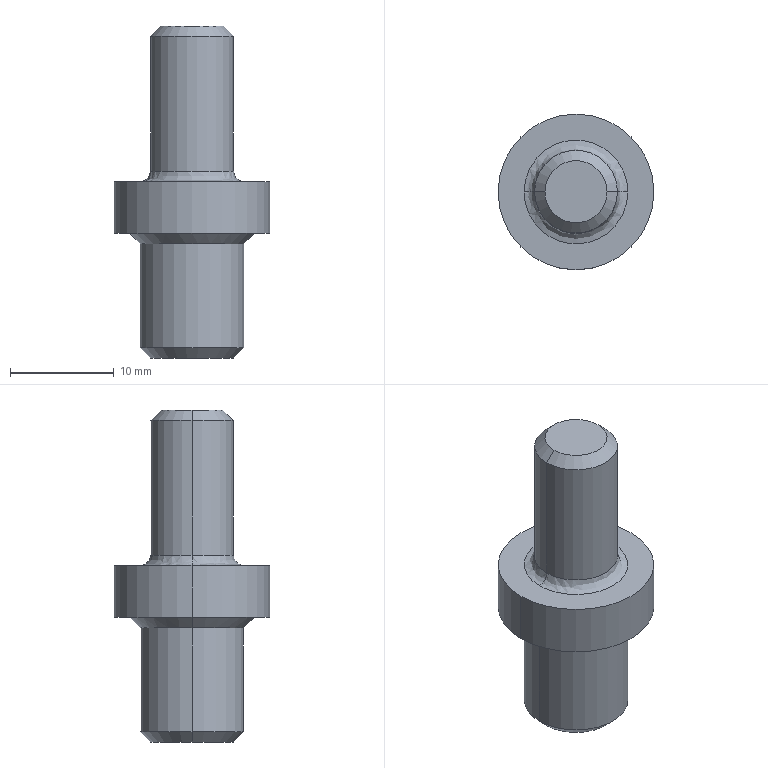Part | SolidWorks | features BaseBody 1 | 1 solid | 18 faces | box 15 x 15 x 32 mm | volume 2576 mm3 | cylinder 6 | cone 6 | plane 4 | spline 2 | commonest cylinder face diameters 8 x2 10 x2 15 x2
STEP:
#1=CARTESIAN_POINT('',(-5.,0.,5.));
#2=VERTEX_POINT('',#1);
#3=CARTESIAN_POINT('',(5.,0.,5.));
#4=VERTEX_POINT('',#3);
#5=CARTESIAN_POINT('',(-5.,0.,5.));
#6=CARTESIAN_POINT('',(-5.,0.3177,5.));
#7=CARTESIAN_POINT('',(-4.956,0.7861,5.));
#8=CARTESIAN_POINT('',(-4.828,1.318,5.));
#9=CARTESIAN_POINT('',(-4.745,1.58,5.));
#10=CARTESIAN_POINT('',(-4.699,1.711,5.));
#11=CARTESIAN_POINT('',(-4.678,1.766,5.));
#12=CARTESIAN_POINT('',(-4.663,1.803,5.));
#13=CARTESIAN_POINT('',(-4.657,1.821,5.));
#14=CARTESIAN_POINT('',(-4.587,1.997,5.));
#15=CARTESIAN_POINT('',(-4.482,2.227,5.));
#16=CARTESIAN_POINT('',(-4.361,2.448,5.));
#17=CARTESIAN_POINT('',(-4.276,2.594,5.));
#18=CARTESIAN_POINT('',(-4.232,2.664,5.));
#19=CARTESIAN_POINT('',(-3.996,3.025,5.));
#20=CARTESIAN_POINT('',(-3.779,3.292,5.));
#21=CARTESIAN_POINT('',(-3.414,3.657,5.));
#22=CARTESIAN_POINT('',(-3.222,3.83,5.));
#23=CARTESIAN_POINT('',(-3.018,3.987,5.));
#24=CARTESIAN_POINT('',(-2.879,4.089,5.));
#25=CARTESIAN_POINT('',(-2.807,4.139,5.));
#26=CARTESIAN_POINT('',(-2.595,4.277,5.));
#27=CARTESIAN_POINT('',(-2.377,4.405,5.));
#28=CARTESIAN_POINT('',(-2.112,4.533,5.));
#29=CARTESIAN_POINT('',(-1.977,4.593,5.));
#30=CARTESIAN_POINT('',(-1.919,4.617,5.));
#31=CARTESIAN_POINT('',(-1.88,4.633,5.));
#32=CARTESIAN_POINT('',(-1.859,4.642,5.));
#33=CARTESIAN_POINT('',(-1.25,4.883,5.));
#34=CARTESIAN_POINT('',(-0.6355,5.,5.));
#35=CARTESIAN_POINT('',(0.3177,5.,5.));
#36=CARTESIAN_POINT('',(0.7861,4.956,5.));
#37=CARTESIAN_POINT('',(1.318,4.828,5.));
#38=CARTESIAN_POINT('',(1.58,4.745,5.));
#39=CARTESIAN_POINT('',(1.711,4.699,5.));
#40=CARTESIAN_POINT('',(1.766,4.678,5.));
#41=CARTESIAN_POINT('',(1.803,4.663,5.));
#42=CARTESIAN_POINT('',(1.821,4.657,5.));
#43=CARTESIAN_POINT('',(1.997,4.587,5.));
#44=CARTESIAN_POINT('',(2.227,4.482,5.));
#45=CARTESIAN_POINT('',(2.448,4.361,5.));
#46=CARTESIAN_POINT('',(2.594,4.276,5.));
#47=CARTESIAN_POINT('',(2.664,4.232,5.));
#48=CARTESIAN_POINT('',(3.025,3.996,5.));
#49=CARTESIAN_POINT('',(3.292,3.779,5.));
#50=CARTESIAN_POINT('',(3.657,3.414,5.));
#51=CARTESIAN_POINT('',(3.83,3.222,5.));
#52=CARTESIAN_POINT('',(3.987,3.018,5.));
#53=CARTESIAN_POINT('',(4.089,2.879,5.));
#54=CARTESIAN_POINT('',(4.139,2.807,5.));
#55=CARTESIAN_POINT('',(4.277,2.595,5.));
#56=CARTESIAN_POINT('',(4.405,2.377,5.));
#57=CARTESIAN_POINT('',(4.533,2.112,5.));
#58=CARTESIAN_POINT('',(4.584,1.996,5.));
#59=CARTESIAN_POINT('',(4.617,1.919,5.));
#60=CARTESIAN_POINT('',(4.634,1.878,5.));
#61=CARTESIAN_POINT('',(4.709,1.69,5.));
#62=CARTESIAN_POINT('',(4.787,1.461,5.));
#63=CARTESIAN_POINT('',(4.858,1.187,5.));
#64=CARTESIAN_POINT('',(4.889,1.049,5.));
#65=CARTESIAN_POINT('',(4.901,0.9894,5.));
#66=CARTESIAN_POINT('',(4.909,0.9497,5.));
#67=CARTESIAN_POINT('',(4.913,0.9286,5.));
#68=CARTESIAN_POINT('',(4.972,0.6093,5.));
#69=CARTESIAN_POINT('',(5.,0.306,5.));
#70=CARTESIAN_POINT('',(5.,0.,5.));
#71=B_SPLINE_CURVE_WITH_KNOTS('',3,(#5,#6,#7,#8,#9,#10,#11,#12,#13,#14,#15,#16,#17,#18,#19,#20,#21,#22,#23,#24,#25,#26,#27,#28,#29,#30,#31,#32,#33,#34,#35,#36,#37,#38,#39,#40,#41,#42,#43,#44,#45,#46,#47,#48,#49,#50,#51,#52,#53,#54,#55,#56,#57,#58,#59,#60,#61,#62,#63,#64,#65,#66,#67,#68,#69,#70),.UNSPECIFIED.,.F.,.F.,(4,1,1,1,1,2,2,1,2,2,2,1,2,2,1,1,1,2,2,2,1,1,1,1,2,2,1,2,2,2,1,2,2,1,1,2,2,1,1,1,2,2,4),(0.5,0.5313,0.5469,0.5547,0.5586,0.5605,0.5625,0.5781,0.5859,0.5938,0.625,0.6406,0.6484,0.6562,0.6719,0.6797,0.6836,0.6855,0.6875,0.75,0.7812,0.7969,0.8047,0.8086,0.8105,0.8125,0.8281,0.8359,0.8437,0.875,0.8906,0.8984,0.9062,0.9219,0.9297,0.9336,0.9375,0.9531,0.9609,0.9648,0.9668,0.9687,1.),.UNSPECIFIED.);
#72=EDGE_CURVE('',#2,#4,#71,.T.);
#73=ORIENTED_EDGE('',*,*,#72,.F.);
#74=CARTESIAN_POINT('',(-4.,0.,6.));
#75=VERTEX_POINT('',#74);
#76=CARTESIAN_POINT('',(-5.,0.,6.));
#77=DIRECTION('',(0.,-1.,0.));
#78=DIRECTION('',(-1.,0.,0.));
#79=AXIS2_PLACEMENT_3D('',#76,#77,#78);
#80=CIRCLE('',#79,1.);
#81=EDGE_CURVE('',#2,#75,#80,.T.);
#82=ORIENTED_EDGE('',*,*,#81,.T.);
#83=CARTESIAN_POINT('',(4.,0.,6.));
#84=VERTEX_POINT('',#83);
#85=CARTESIAN_POINT('',(0.,0.,6.));
#86=DIRECTION('',(0.,0.,1.));
#87=DIRECTION('',(-1.,0.,0.));
#88=AXIS2_PLACEMENT_3D('',#85,#86,#87);
#89=CIRCLE('',#88,4.);
#90=EDGE_CURVE('',#84,#75,#89,.T.);
#91=ORIENTED_EDGE('',*,*,#90,.F.);
#92=CARTESIAN_POINT('',(5.,0.,6.));
#93=DIRECTION('',(0.,1.,0.));
#94=DIRECTION('',(1.,0.,0.));
#95=AXIS2_PLACEMENT_3D('',#92,#93,#94);
#96=CIRCLE('',#95,1.);
#97=EDGE_CURVE('',#4,#84,#96,.T.);
#98=ORIENTED_EDGE('',*,*,#97,.F.);
#99=EDGE_LOOP('',(#73,#82,#91,#98));
#100=FACE_OUTER_BOUND('',#99,.T.);
#101=CARTESIAN_POINT('',(5.,0.,5.));
#102=CARTESIAN_POINT('',(5.,10.,5.));
#103=CARTESIAN_POINT('',(-5.,10.,5.));
#104=CARTESIAN_POINT('',(-5.,0.,5.));
#105=CARTESIAN_POINT('',(4.414,0.,5.));
#106=CARTESIAN_POINT('',(4.414,8.828,5.));
#107=CARTESIAN_POINT('',(-4.414,8.828,5.));
#108=CARTESIAN_POINT('',(-4.414,0.,5.));
#109=CARTESIAN_POINT('',(4.,0.,5.414));
#110=CARTESIAN_POINT('',(4.,8.,5.414));
#111=CARTESIAN_POINT('',(-4.,8.,5.414));
#112=CARTESIAN_POINT('',(-4.,0.,5.414));
#113=CARTESIAN_POINT('',(4.,0.,6.));
#114=CARTESIAN_POINT('',(4.,8.,6.));
#115=CARTESIAN_POINT('',(-4.,8.,6.));
#116=CARTESIAN_POINT('',(-4.,0.,6.));
#117=(BOUNDED_SURFACE()B_SPLINE_SURFACE(3,3,((#101,#102,#103,#104),(#105,#106,#107,#108),(#109,#110,#111,#112),(#113,#114,#115,#116)),.UNSPECIFIED.,.F.,.F.,.F.)B_SPLINE_SURFACE_WITH_KNOTS((4,4),(4,4),(0.,1.),(0.,1.),.UNSPECIFIED.)GEOMETRIC_REPRESENTATION_ITEM()RATIONAL_B_SPLINE_SURFACE(((1.,0.3333,0.3333,1.),(0.8047,0.2682,0.2682,0.8047),(0.8047,0.2682,0.2682,0.8047),(1.,0.3333,0.3333,1.)))REPRESENTATION_ITEM('')SURFACE());
#118=ADVANCED_FACE('',(#100),#117,.F.);
#119=CARTESIAN_POINT('',(-4.,0.,19.));
#120=VERTEX_POINT('',#119);
#121=CARTESIAN_POINT('',(4.,0.,19.));
#122=VERTEX_POINT('',#121);
#123=CARTESIAN_POINT('',(0.,0.,19.));
#124=DIRECTION('',(0.,0.,-1.));
#125=DIRECTION('',(-1.,0.,0.));
#126=AXIS2_PLACEMENT_3D('',#123,#124,#125);
#127=CIRCLE('',#126,4.);
#128=EDGE_CURVE('',#120,#122,#127,.T.);
#129=ORIENTED_EDGE('',*,*,#128,.T.);
#130=CARTESIAN_POINT('',(4.,0.,20.));
#131=DIRECTION('',(0.,0.,-1.));
#132=VECTOR('',#131,1000.);
#133=LINE('',#130,#132);
#134=EDGE_CURVE('',#122,#84,#133,.T.);
#135=ORIENTED_EDGE('',*,*,#134,.T.);
#136=ORIENTED_EDGE('',*,*,#90,.T.);
#137=CARTESIAN_POINT('',(-4.,0.,20.));
#138=DIRECTION('',(0.,0.,-1.));
#139=VECTOR('',#138,1000.);
#140=LINE('',#137,#139);
#141=EDGE_CURVE('',#120,#75,#140,.T.);
#142=ORIENTED_EDGE('',*,*,#141,.F.);
#143=EDGE_LOOP('',(#129,#135,#136,#142));
#144=FACE_OUTER_BOUND('',#143,.T.);
#145=CARTESIAN_POINT('',(0.,0.,20.));
#146=DIRECTION('',(0.,0.,-1.));
#147=DIRECTION('',(-1.,0.,0.));
#148=AXIS2_PLACEMENT_3D('',#145,#146,#147);
#149=CYLINDRICAL_SURFACE('',#148,4.);
#150=ADVANCED_FACE('',(#144),#149,.T.);
#151=CARTESIAN_POINT('',(-3.,0.,20.));
#152=VERTEX_POINT('',#151);
#153=CARTESIAN_POINT('',(3.,0.,20.));
#154=VERTEX_POINT('',#153);
#155=CARTESIAN_POINT('',(0.,0.,20.));
#156=DIRECTION('',(0.,0.,-1.));
#157=DIRECTION('',(-1.,0.,0.));
#158=AXIS2_PLACEMENT_3D('',#155,#156,#157);
#159=CIRCLE('',#158,3.);
#160=EDGE_CURVE('',#152,#154,#159,.T.);
#161=ORIENTED_EDGE('',*,*,#160,.T.);
#162=CARTESIAN_POINT('',(4.,0.,19.));
#163=DIRECTION('',(0.7071,0.,-0.7071));
#164=VECTOR('',#163,1000.);
#165=LINE('',#162,#164);
#166=EDGE_CURVE('',#154,#122,#165,.T.);
#167=ORIENTED_EDGE('',*,*,#166,.T.);
#168=ORIENTED_EDGE('',*,*,#128,.F.);
#169=CARTESIAN_POINT('',(-4.,0.,19.));
#170=DIRECTION('',(-0.7071,0.,-0.7071));
#171=VECTOR('',#170,1000.);
#172=LINE('',#169,#171);
#173=EDGE_CURVE('',#152,#120,#172,.T.);
#174=ORIENTED_EDGE('',*,*,#173,.F.);
#175=EDGE_LOOP('',(#161,#167,#168,#174));
#176=FACE_OUTER_BOUND('',#175,.T.);
#177=CARTESIAN_POINT('',(0.,0.,19.));
#178=DIRECTION('',(0.,0.,-1.));
#179=DIRECTION('',(-1.,0.,0.));
#180=AXIS2_PLACEMENT_3D('',#177,#178,#179);
#181=CONICAL_SURFACE('',#180,4.,0.7854);
#182=ADVANCED_FACE('',(#176),#181,.T.);
#183=CARTESIAN_POINT('',(7.5,0.,5.));
#184=VERTEX_POINT('',#183);
#185=CARTESIAN_POINT('',(-7.5,0.,5.));
#186=VERTEX_POINT('',#185);
#187=CARTESIAN_POINT('',(0.,0.,5.));
#188=DIRECTION('',(0.,0.,1.));
#189=DIRECTION('',(-1.,0.,0.));
#190=AXIS2_PLACEMENT_3D('',#187,#188,#189);
#191=CIRCLE('',#190,7.5);
#192=EDGE_CURVE('',#184,#186,#191,.T.);
#193=ORIENTED_EDGE('',*,*,#192,.F.);
#194=CARTESIAN_POINT('',(7.5,0.,0.));
#195=VERTEX_POINT('',#194);
#196=CARTESIAN_POINT('',(7.5,0.,5.));
#197=DIRECTION('',(0.,0.,-1.));
#198=VECTOR('',#197,1000.);
#199=LINE('',#196,#198);
#200=EDGE_CURVE('',#184,#195,#199,.T.);
#201=ORIENTED_EDGE('',*,*,#200,.T.);
#202=CARTESIAN_POINT('',(-7.5,0.,0.));
#203=VERTEX_POINT('',#202);
#204=CARTESIAN_POINT('',(0.,0.,0.));
#205=DIRECTION('',(0.,0.,1.));
#206=DIRECTION('',(-1.,0.,0.));
#207=AXIS2_PLACEMENT_3D('',#204,#205,#206);
#208=CIRCLE('',#207,7.5);
#209=EDGE_CURVE('',#195,#203,#208,.T.);
#210=ORIENTED_EDGE('',*,*,#209,.T.);
#211=CARTESIAN_POINT('',(-7.5,0.,5.));
#212=DIRECTION('',(0.,0.,-1.));
#213=VECTOR('',#212,1000.);
#214=LINE('',#211,#213);
#215=EDGE_CURVE('',#186,#203,#214,.T.);
#216=ORIENTED_EDGE('',*,*,#215,.F.);
#217=EDGE_LOOP('',(#193,#201,#210,#216));
#218=FACE_OUTER_BOUND('',#217,.T.);
#219=CARTESIAN_POINT('',(0.,0.,5.));
#220=DIRECTION('',(0.,0.,-1.));
#221=DIRECTION('',(-1.,0.,0.));
#222=AXIS2_PLACEMENT_3D('',#219,#220,#221);
#223=CYLINDRICAL_SURFACE('',#222,7.5);
#224=ADVANCED_FACE('',(#218),#223,.T.);
#225=CARTESIAN_POINT('',(5.,0.,-1.));
#226=VERTEX_POINT('',#225);
#227=CARTESIAN_POINT('',(-5.,0.,-1.));
#228=VERTEX_POINT('',#227);
#229=CARTESIAN_POINT('',(0.,0.,-1.));
#230=DIRECTION('',(0.,0.,1.));
#231=DIRECTION('',(1.,0.,0.));
#232=AXIS2_PLACEMENT_3D('',#229,#230,#231);
#233=CIRCLE('',#232,5.);
#234=EDGE_CURVE('',#226,#228,#233,.T.);
#235=ORIENTED_EDGE('',*,*,#234,.T.);
#236=CARTESIAN_POINT('',(-6.,0.,0.));
#237=VERTEX_POINT('',#236);
#238=CARTESIAN_POINT('',(-6.,0.,0.));
#239=DIRECTION('',(-0.7071,0.,0.7071));
#240=VECTOR('',#239,1000.);
#241=LINE('',#238,#240);
#242=EDGE_CURVE('',#228,#237,#241,.T.);
#243=ORIENTED_EDGE('',*,*,#242,.T.);
#244=CARTESIAN_POINT('',(6.,0.,0.));
#245=VERTEX_POINT('',#244);
#246=CARTESIAN_POINT('',(0.,0.,0.));
#247=DIRECTION('',(0.,0.,-1.));
#248=DIRECTION('',(1.,0.,0.));
#249=AXIS2_PLACEMENT_3D('',#246,#247,#248);
#250=CIRCLE('',#249,6.);
#251=EDGE_CURVE('',#237,#245,#250,.T.);
#252=ORIENTED_EDGE('',*,*,#251,.T.);
#253=CARTESIAN_POINT('',(6.,0.,0.));
#254=DIRECTION('',(0.7071,0.,0.7071));
#255=VECTOR('',#254,1000.);
#256=LINE('',#253,#255);
#257=EDGE_CURVE('',#226,#245,#256,.T.);
#258=ORIENTED_EDGE('',*,*,#257,.F.);
#259=EDGE_LOOP('',(#235,#243,#252,#258));
#260=FACE_OUTER_BOUND('',#259,.T.);
#261=CARTESIAN_POINT('',(0.,0.,0.));
#262=DIRECTION('',(0.,0.,1.));
#263=DIRECTION('',(1.,0.,0.));
#264=AXIS2_PLACEMENT_3D('',#261,#262,#263);
#265=CONICAL_SURFACE('',#264,6.,0.7854);
#266=ADVANCED_FACE('',(#260),#265,.T.);
#267=CARTESIAN_POINT('',(5.,0.,-11.));
#268=VERTEX_POINT('',#267);
#269=CARTESIAN_POINT('',(-5.,0.,-11.));
#270=VERTEX_POINT('',#269);
#271=CARTESIAN_POINT('',(0.,0.,-11.));
#272=DIRECTION('',(0.,0.,1.));
#273=DIRECTION('',(1.,0.,0.));
#274=AXIS2_PLACEMENT_3D('',#271,#272,#273);
#275=CIRCLE('',#274,5.);
#276=EDGE_CURVE('',#268,#270,#275,.T.);
#277=ORIENTED_EDGE('',*,*,#276,.T.);
#278=CARTESIAN_POINT('',(-5.,0.,-12.));
#279=DIRECTION('',(0.,0.,1.));
#280=VECTOR('',#279,1000.);
#281=LINE('',#278,#280);
#282=EDGE_CURVE('',#270,#228,#281,.T.);
#283=ORIENTED_EDGE('',*,*,#282,.T.);
#284=ORIENTED_EDGE('',*,*,#234,.F.);
#285=CARTESIAN_POINT('',(5.,0.,-12.));
#286=DIRECTION('',(0.,0.,1.));
#287=VECTOR('',#286,1000.);
#288=LINE('',#285,#287);
#289=EDGE_CURVE('',#268,#226,#288,.T.);
#290=ORIENTED_EDGE('',*,*,#289,.F.);
#291=EDGE_LOOP('',(#277,#283,#284,#290));
#292=FACE_OUTER_BOUND('',#291,.T.);
#293=CARTESIAN_POINT('',(0.,0.,-12.));
#294=DIRECTION('',(0.,0.,1.));
#295=DIRECTION('',(1.,0.,0.));
#296=AXIS2_PLACEMENT_3D('',#293,#294,#295);
#297=CYLINDRICAL_SURFACE('',#296,5.);
#298=ADVANCED_FACE('',(#292),#297,.T.);
#299=CARTESIAN_POINT('',(4.,0.,-12.));
#300=VERTEX_POINT('',#299);
#301=CARTESIAN_POINT('',(-4.,0.,-12.));
#302=VERTEX_POINT('',#301);
#303=CARTESIAN_POINT('',(0.,0.,-12.));
#304=DIRECTION('',(0.,0.,1.));
#305=DIRECTION('',(1.,0.,0.));
#306=AXIS2_PLACEMENT_3D('',#303,#304,#305);
#307=CIRCLE('',#306,4.);
#308=EDGE_CURVE('',#300,#302,#307,.T.);
#309=ORIENTED_EDGE('',*,*,#308,.T.);
#310=CARTESIAN_POINT('',(-5.,0.,-11.));
#311=DIRECTION('',(-0.7071,0.,0.7071));
#312=VECTOR('',#311,1000.);
#313=LINE('',#310,#312);
#314=EDGE_CURVE('',#302,#270,#313,.T.);
#315=ORIENTED_EDGE('',*,*,#314,.T.);
#316=ORIENTED_EDGE('',*,*,#276,.F.);
#317=CARTESIAN_POINT('',(5.,0.,-11.));
#318=DIRECTION('',(0.7071,0.,0.7071));
#319=VECTOR('',#318,1000.);
#320=LINE('',#317,#319);
#321=EDGE_CURVE('',#300,#268,#320,.T.);
#322=ORIENTED_EDGE('',*,*,#321,.F.);
#323=EDGE_LOOP('',(#309,#315,#316,#322));
#324=FACE_OUTER_BOUND('',#323,.T.);
#325=CARTESIAN_POINT('',(0.,0.,-11.));
#326=DIRECTION('',(0.,0.,1.));
#327=DIRECTION('',(1.,0.,0.));
#328=AXIS2_PLACEMENT_3D('',#325,#326,#327);
#329=CONICAL_SURFACE('',#328,5.,0.7854);
#330=ADVANCED_FACE('',(#324),#329,.T.);
#331=ORIENTED_EDGE('',*,*,#134,.F.);
#332=CARTESIAN_POINT('',(0.,0.,19.));
#333=DIRECTION('',(0.,0.,-1.));
#334=DIRECTION('',(-1.,0.,0.));
#335=AXIS2_PLACEMENT_3D('',#332,#333,#334);
#336=CIRCLE('',#335,4.);
#337=EDGE_CURVE('',#122,#120,#336,.T.);
#338=ORIENTED_EDGE('',*,*,#337,.T.);
#339=ORIENTED_EDGE('',*,*,#141,.T.);
#340=CARTESIAN_POINT('',(0.,0.,6.));
#341=DIRECTION('',(0.,0.,1.));
#342=DIRECTION('',(-1.,0.,0.));
#343=AXIS2_PLACEMENT_3D('',#340,#341,#342);
#344=CIRCLE('',#343,4.);
#345=EDGE_CURVE('',#75,#84,#344,.T.);
#346=ORIENTED_EDGE('',*,*,#345,.T.);
#347=EDGE_LOOP('',(#331,#338,#339,#346));
#348=FACE_OUTER_BOUND('',#347,.T.);
#349=CARTESIAN_POINT('',(0.,0.,20.));
#350=DIRECTION('',(0.,0.,-1.));
#351=DIRECTION('',(-1.,0.,0.));
#352=AXIS2_PLACEMENT_3D('',#349,#350,#351);
#353=CYLINDRICAL_SURFACE('',#352,4.);
#354=ADVANCED_FACE('',(#348),#353,.T.);
#355=ORIENTED_EDGE('',*,*,#81,.F.);
#356=CARTESIAN_POINT('',(5.,0.,5.));
#357=CARTESIAN_POINT('',(5.,-0.3178,5.));
#358=CARTESIAN_POINT('',(4.956,-0.7862,5.));
#359=CARTESIAN_POINT('',(4.828,-1.318,5.));
#360=CARTESIAN_POINT('',(4.745,-1.581,5.));
#361=CARTESIAN_POINT('',(4.699,-1.711,5.));
#362=CARTESIAN_POINT('',(4.678,-1.766,5.));
#363=CARTESIAN_POINT('',(4.663,-1.803,5.));
#364=CARTESIAN_POINT('',(4.657,-1.821,5.));
#365=CARTESIAN_POINT('',(4.587,-1.997,5.));
#366=CARTESIAN_POINT('',(4.482,-2.227,5.));
#367=CARTESIAN_POINT('',(4.361,-2.448,5.));
#368=CARTESIAN_POINT('',(4.276,-2.594,5.));
#369=CARTESIAN_POINT('',(4.232,-2.664,5.));
#370=CARTESIAN_POINT('',(3.996,-3.025,5.));
#371=CARTESIAN_POINT('',(3.779,-3.292,5.));
#372=CARTESIAN_POINT('',(3.414,-3.657,5.));
#373=CARTESIAN_POINT('',(3.222,-3.83,5.));
#374=CARTESIAN_POINT('',(3.018,-3.987,5.));
#375=CARTESIAN_POINT('',(2.879,-4.089,5.));
#376=CARTESIAN_POINT('',(2.807,-4.139,5.));
#377=CARTESIAN_POINT('',(2.595,-4.277,5.));
#378=CARTESIAN_POINT('',(2.377,-4.405,5.));
#379=CARTESIAN_POINT('',(2.112,-4.533,5.));
#380=CARTESIAN_POINT('',(1.977,-4.593,5.));
#381=CARTESIAN_POINT('',(1.919,-4.617,5.));
#382=CARTESIAN_POINT('',(1.88,-4.633,5.));
#383=CARTESIAN_POINT('',(1.859,-4.642,5.));
#384=CARTESIAN_POINT('',(1.25,-4.883,5.));
#385=CARTESIAN_POINT('',(0.6355,-5.,5.));
#386=CARTESIAN_POINT('',(-0.3177,-5.,5.));
#387=CARTESIAN_POINT('',(-0.7861,-4.956,5.));
#388=CARTESIAN_POINT('',(-1.318,-4.828,5.));
#389=CARTESIAN_POINT('',(-1.58,-4.745,5.));
#390=CARTESIAN_POINT('',(-1.711,-4.699,5.));
#391=CARTESIAN_POINT('',(-1.766,-4.678,5.));
#392=CARTESIAN_POINT('',(-1.803,-4.663,5.));
#393=CARTESIAN_POINT('',(-1.821,-4.657,5.));
#394=CARTESIAN_POINT('',(-1.997,-4.587,5.));
#395=CARTESIAN_POINT('',(-2.227,-4.482,5.));
#396=CARTESIAN_POINT('',(-2.448,-4.361,5.));
#397=CARTESIAN_POINT('',(-2.594,-4.276,5.));
#398=CARTESIAN_POINT('',(-2.664,-4.232,5.));
#399=CARTESIAN_POINT('',(-3.025,-3.996,5.));
#400=CARTESIAN_POINT('',(-3.292,-3.779,5.));
#401=CARTESIAN_POINT('',(-3.657,-3.414,5.));
#402=CARTESIAN_POINT('',(-3.83,-3.222,5.));
#403=CARTESIAN_POINT('',(-3.987,-3.018,5.));
#404=CARTESIAN_POINT('',(-4.089,-2.879,5.));
#405=CARTESIAN_POINT('',(-4.139,-2.807,5.));
#406=CARTESIAN_POINT('',(-4.277,-2.595,5.));
#407=CARTESIAN_POINT('',(-4.405,-2.377,5.));
#408=CARTESIAN_POINT('',(-4.533,-2.112,5.));
#409=CARTESIAN_POINT('',(-4.593,-1.977,5.));
#410=CARTESIAN_POINT('',(-4.617,-1.919,5.));
#411=CARTESIAN_POINT('',(-4.633,-1.88,5.));
#412=CARTESIAN_POINT('',(-4.642,-1.859,5.));
#413=CARTESIAN_POINT('',(-4.883,-1.25,5.));
#414=CARTESIAN_POINT('',(-5.,-0.6355,5.));
#415=CARTESIAN_POINT('',(-5.,0.,5.));
#416=B_SPLINE_CURVE_WITH_KNOTS('',3,(#356,#357,#358,#359,#360,#361,#362,#363,#364,#365,#366,#367,#368,#369,#370,#371,#372,#373,#374,#375,#376,#377,#378,#379,#380,#381,#382,#383,#384,#385,#386,#387,#388,#389,#390,#391,#392,#393,#394,#395,#396,#397,#398,#399,#400,#401,#402,#403,#404,#405,#406,#407,#408,#409,#410,#411,#412,#413,#414,#415),.UNSPECIFIED.,.F.,.F.,(4,1,1,1,1,2,2,1,2,2,2,1,2,2,1,1,1,2,2,2,1,1,1,1,2,2,1,2,2,2,1,2,2,1,1,1,2,2,4),(0.,0.03125,0.04687,0.05469,0.05859,0.06055,0.0625,0.07812,0.08594,0.09375,0.125,0.1406,0.1484,0.1562,0.1719,0.1797,0.1836,0.1855,0.1875,0.25,0.2812,0.2969,0.3047,0.3086,0.3105,0.3125,0.3281,0.3359,0.3437,0.375,0.3906,0.3984,0.4062,0.4219,0.4297,0.4336,0.4355,0.4375,0.5),.UNSPECIFIED.);
#417=EDGE_CURVE('',#4,#2,#416,.T.);
#418=ORIENTED_EDGE('',*,*,#417,.F.);
#419=ORIENTED_EDGE('',*,*,#97,.T.);
#420=ORIENTED_EDGE('',*,*,#345,.F.);
#421=EDGE_LOOP('',(#355,#418,#419,#420));
#422=FACE_OUTER_BOUND('',#421,.T.);
#423=CARTESIAN_POINT('',(-5.,0.,5.));
#424=CARTESIAN_POINT('',(-5.,-10.,5.));
#425=CARTESIAN_POINT('',(5.,-10.,5.));
#426=CARTESIAN_POINT('',(5.,0.,5.));
#427=CARTESIAN_POINT('',(-4.414,0.,5.));
#428=CARTESIAN_POINT('',(-4.414,-8.828,5.));
#429=CARTESIAN_POINT('',(4.414,-8.828,5.));
#430=CARTESIAN_POINT('',(4.414,0.,5.));
#431=CARTESIAN_POINT('',(-4.,0.,5.414));
#432=CARTESIAN_POINT('',(-4.,-8.,5.414));
#433=CARTESIAN_POINT('',(4.,-8.,5.414));
#434=CARTESIAN_POINT('',(4.,0.,5.414));
#435=CARTESIAN_POINT('',(-4.,0.,6.));
#436=CARTESIAN_POINT('',(-4.,-8.,6.));
#437=CARTESIAN_POINT('',(4.,-8.,6.));
#438=CARTESIAN_POINT('',(4.,0.,6.));
#439=(BOUNDED_SURFACE()B_SPLINE_SURFACE(3,3,((#423,#424,#425,#426),(#427,#428,#429,#430),(#431,#432,#433,#434),(#435,#436,#437,#438)),.UNSPECIFIED.,.F.,.F.,.T.)B_SPLINE_SURFACE_WITH_KNOTS((4,4),(4,4),(0.,1.),(0.,1.),.UNSPECIFIED.)GEOMETRIC_REPRESENTATION_ITEM()RATIONAL_B_SPLINE_SURFACE(((1.,0.3333,0.3333,1.),(0.8047,0.2682,0.2682,0.8047),(0.8047,0.2682,0.2682,0.8047),(1.,0.3333,0.3333,1.)))REPRESENTATION_ITEM('')SURFACE());
#440=ADVANCED_FACE('',(#422),#439,.F.);
#441=ORIENTED_EDGE('',*,*,#166,.F.);
#442=CARTESIAN_POINT('',(0.,0.,20.));
#443=DIRECTION('',(0.,0.,-1.));
#444=DIRECTION('',(-1.,0.,0.));
#445=AXIS2_PLACEMENT_3D('',#442,#443,#444);
#446=CIRCLE('',#445,3.);
#447=EDGE_CURVE('',#154,#152,#446,.T.);
#448=ORIENTED_EDGE('',*,*,#447,.T.);
#449=ORIENTED_EDGE('',*,*,#173,.T.);
#450=ORIENTED_EDGE('',*,*,#337,.F.);
#451=EDGE_LOOP('',(#441,#448,#449,#450));
#452=FACE_OUTER_BOUND('',#451,.T.);
#453=CARTESIAN_POINT('',(0.,0.,19.));
#454=DIRECTION('',(0.,0.,-1.));
#455=DIRECTION('',(-1.,0.,0.));
#456=AXIS2_PLACEMENT_3D('',#453,#454,#455);
#457=CONICAL_SURFACE('',#456,4.,0.7854);
#458=ADVANCED_FACE('',(#452),#457,.T.);
#459=CARTESIAN_POINT('',(0.,0.,5.));
#460=DIRECTION('',(0.,0.,1.));
#461=DIRECTION('',(-1.,0.,0.));
#462=AXIS2_PLACEMENT_3D('',#459,#460,#461);
#463=CIRCLE('',#462,7.5);
#464=EDGE_CURVE('',#186,#184,#463,.T.);
#465=ORIENTED_EDGE('',*,*,#464,.T.);
#466=ORIENTED_EDGE('',*,*,#192,.T.);
#467=EDGE_LOOP('',(#465,#466));
#468=FACE_OUTER_BOUND('',#467,.T.);
#469=ORIENTED_EDGE('',*,*,#417,.T.);
#470=ORIENTED_EDGE('',*,*,#72,.T.);
#471=EDGE_LOOP('',(#469,#470));
#472=FACE_BOUND('',#471,.T.);
#473=CARTESIAN_POINT('',(0.,0.,5.));
#474=DIRECTION('',(0.,0.,1.));
#475=DIRECTION('',(1.,0.,0.));
#476=AXIS2_PLACEMENT_3D('',#473,#474,#475);
#477=PLANE('',#476);
#478=ADVANCED_FACE('',(#468,#472),#477,.T.);
#479=ORIENTED_EDGE('',*,*,#160,.F.);
#480=ORIENTED_EDGE('',*,*,#447,.F.);
#481=EDGE_LOOP('',(#479,#480));
#482=FACE_OUTER_BOUND('',#481,.T.);
#483=CARTESIAN_POINT('',(0.,0.,20.));
#484=DIRECTION('',(0.,0.,-1.));
#485=DIRECTION('',(-1.,0.,0.));
#486=AXIS2_PLACEMENT_3D('',#483,#484,#485);
#487=PLANE('',#486);
#488=ADVANCED_FACE('',(#482),#487,.F.);
#489=ORIENTED_EDGE('',*,*,#200,.F.);
#490=ORIENTED_EDGE('',*,*,#464,.F.);
#491=ORIENTED_EDGE('',*,*,#215,.T.);
#492=CARTESIAN_POINT('',(0.,0.,0.));
#493=DIRECTION('',(0.,0.,1.));
#494=DIRECTION('',(-1.,0.,0.));
#495=AXIS2_PLACEMENT_3D('',#492,#493,#494);
#496=CIRCLE('',#495,7.5);
#497=EDGE_CURVE('',#203,#195,#496,.T.);
#498=ORIENTED_EDGE('',*,*,#497,.T.);
#499=EDGE_LOOP('',(#489,#490,#491,#498));
#500=FACE_OUTER_BOUND('',#499,.T.);
#501=CARTESIAN_POINT('',(0.,0.,5.));
#502=DIRECTION('',(0.,0.,-1.));
#503=DIRECTION('',(-1.,0.,0.));
#504=AXIS2_PLACEMENT_3D('',#501,#502,#503);
#505=CYLINDRICAL_SURFACE('',#504,7.5);
#506=ADVANCED_FACE('',(#500),#505,.T.);
#507=ORIENTED_EDGE('',*,*,#497,.F.);
#508=ORIENTED_EDGE('',*,*,#209,.F.);
#509=EDGE_LOOP('',(#507,#508));
#510=FACE_OUTER_BOUND('',#509,.T.);
#511=CARTESIAN_POINT('',(0.,0.,0.));
#512=DIRECTION('',(0.,0.,-1.));
#513=DIRECTION('',(1.,0.,0.));
#514=AXIS2_PLACEMENT_3D('',#511,#512,#513);
#515=CIRCLE('',#514,6.);
#516=EDGE_CURVE('',#245,#237,#515,.T.);
#517=ORIENTED_EDGE('',*,*,#516,.F.);
#518=ORIENTED_EDGE('',*,*,#251,.F.);
#519=EDGE_LOOP('',(#517,#518));
#520=FACE_BOUND('',#519,.T.);
#521=CARTESIAN_POINT('',(0.,0.,0.));
#522=DIRECTION('',(0.,0.,1.));
#523=DIRECTION('',(1.,0.,0.));
#524=AXIS2_PLACEMENT_3D('',#521,#522,#523);
#525=PLANE('',#524);
#526=ADVANCED_FACE('',(#510,#520),#525,.F.);
#527=ORIENTED_EDGE('',*,*,#242,.F.);
#528=CARTESIAN_POINT('',(0.,0.,-1.));
#529=DIRECTION('',(0.,0.,1.));
#530=DIRECTION('',(1.,0.,0.));
#531=AXIS2_PLACEMENT_3D('',#528,#529,#530);
#532=CIRCLE('',#531,5.);
#533=EDGE_CURVE('',#228,#226,#532,.T.);
#534=ORIENTED_EDGE('',*,*,#533,.T.);
#535=ORIENTED_EDGE('',*,*,#257,.T.);
#536=ORIENTED_EDGE('',*,*,#516,.T.);
#537=EDGE_LOOP('',(#527,#534,#535,#536));
#538=FACE_OUTER_BOUND('',#537,.T.);
#539=CARTESIAN_POINT('',(0.,0.,0.));
#540=DIRECTION('',(0.,0.,1.));
#541=DIRECTION('',(1.,0.,0.));
#542=AXIS2_PLACEMENT_3D('',#539,#540,#541);
#543=CONICAL_SURFACE('',#542,6.,0.7854);
#544=ADVANCED_FACE('',(#538),#543,.T.);
#545=ORIENTED_EDGE('',*,*,#282,.F.);
#546=CARTESIAN_POINT('',(0.,0.,-11.));
#547=DIRECTION('',(0.,0.,1.));
#548=DIRECTION('',(1.,0.,0.));
#549=AXIS2_PLACEMENT_3D('',#546,#547,#548);
#550=CIRCLE('',#549,5.);
#551=EDGE_CURVE('',#270,#268,#550,.T.);
#552=ORIENTED_EDGE('',*,*,#551,.T.);
#553=ORIENTED_EDGE('',*,*,#289,.T.);
#554=ORIENTED_EDGE('',*,*,#533,.F.);
#555=EDGE_LOOP('',(#545,#552,#553,#554));
#556=FACE_OUTER_BOUND('',#555,.T.);
#557=CARTESIAN_POINT('',(0.,0.,-12.));
#558=DIRECTION('',(0.,0.,1.));
#559=DIRECTION('',(1.,0.,0.));
#560=AXIS2_PLACEMENT_3D('',#557,#558,#559);
#561=CYLINDRICAL_SURFACE('',#560,5.);
#562=ADVANCED_FACE('',(#556),#561,.T.);
#563=ORIENTED_EDGE('',*,*,#314,.F.);
#564=CARTESIAN_POINT('',(0.,0.,-12.));
#565=DIRECTION('',(0.,0.,1.));
#566=DIRECTION('',(1.,0.,0.));
#567=AXIS2_PLACEMENT_3D('',#564,#565,#566);
#568=CIRCLE('',#567,4.);
#569=EDGE_CURVE('',#302,#300,#568,.T.);
#570=ORIENTED_EDGE('',*,*,#569,.T.);
#571=ORIENTED_EDGE('',*,*,#321,.T.);
#572=ORIENTED_EDGE('',*,*,#551,.F.);
#573=EDGE_LOOP('',(#563,#570,#571,#572));
#574=FACE_OUTER_BOUND('',#573,.T.);
#575=CARTESIAN_POINT('',(0.,0.,-11.));
#576=DIRECTION('',(0.,0.,1.));
#577=DIRECTION('',(1.,0.,0.));
#578=AXIS2_PLACEMENT_3D('',#575,#576,#577);
#579=CONICAL_SURFACE('',#578,5.,0.7854);
#580=ADVANCED_FACE('',(#574),#579,.T.);
#581=ORIENTED_EDGE('',*,*,#308,.F.);
#582=ORIENTED_EDGE('',*,*,#569,.F.);
#583=EDGE_LOOP('',(#581,#582));
#584=FACE_OUTER_BOUND('',#583,.T.);
#585=CARTESIAN_POINT('',(0.,0.,-12.));
#586=DIRECTION('',(0.,0.,1.));
#587=DIRECTION('',(1.,0.,0.));
#588=AXIS2_PLACEMENT_3D('',#585,#586,#587);
#589=PLANE('',#588);
#590=ADVANCED_FACE('',(#584),#589,.F.);
#591=CLOSED_SHELL('',(#118,#150,#182,#224,#266,#298,#330,#354,#440,#458,#478,#488,#506,#526,#544,#562,#580,#590));
#592=MANIFOLD_SOLID_BREP('',#591);
#593=CARTESIAN_POINT('',(0.,0.,0.));
#594=DIRECTION('',(0.,0.,1.));
#595=DIRECTION('',(1.,0.,0.));
#596=AXIS2_PLACEMENT_3D('',#593,#594,#595);
#597=(LENGTH_UNIT()NAMED_UNIT(*)SI_UNIT(.MILLI.,.METRE.));
#598=UNCERTAINTY_MEASURE_WITH_UNIT(LENGTH_MEASURE(0.00001),#597,'','');
#599=(NAMED_UNIT(*)PLANE_ANGLE_UNIT()SI_UNIT($,.RADIAN.));
#600=(NAMED_UNIT(*)SI_UNIT($,.STERADIAN.)SOLID_ANGLE_UNIT());
#601=(GEOMETRIC_REPRESENTATION_CONTEXT(3)GLOBAL_UNCERTAINTY_ASSIGNED_CONTEXT((#598))GLOBAL_UNIT_ASSIGNED_CONTEXT((#597,#599,#600))REPRESENTATION_CONTEXT('',''));
#602=ADVANCED_BREP_SHAPE_REPRESENTATION('',(#592,#596),#601);